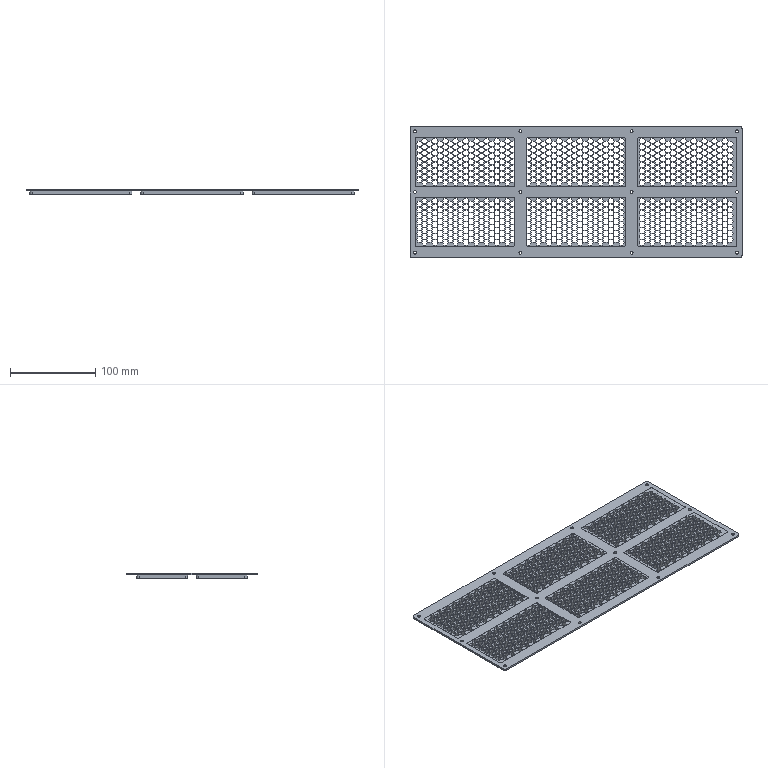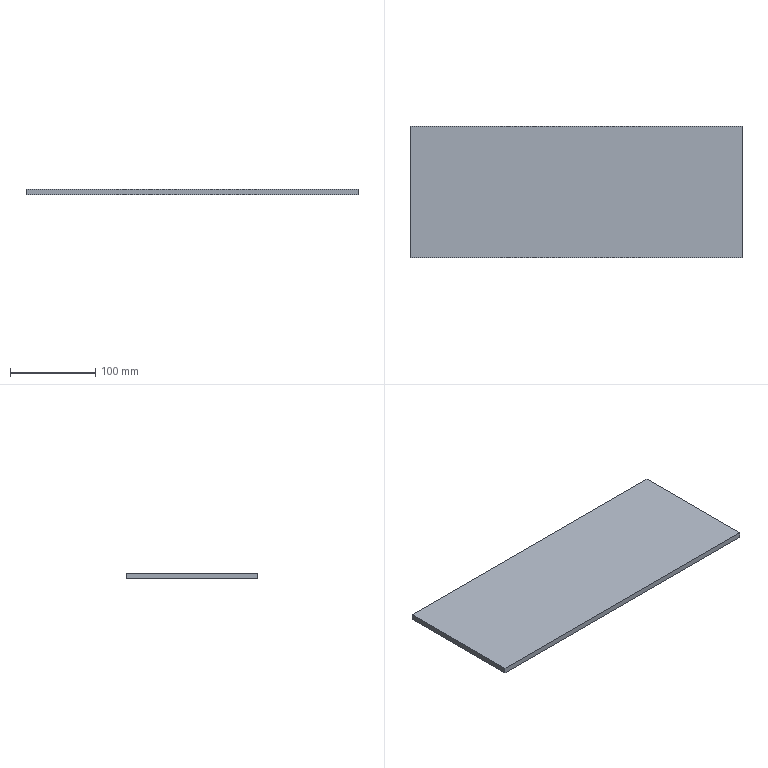CAM job | NX | 3-axis milling, drilling | stock box 388.5 x 153.5 x 6.5 mm
Tools:
number,name,description,diameter,corner_radius,flute_length,length,flutes
3,D2_FINISH,D2,2.0,0.0,6.0,50.0,2
12,D3_ROUGH,D3,3.0,0.0,9.0,50.0,2
0,D4_ROUGH,D4,4.0,0.0,12.0,50.0,2
2,D6_ROUGH,D6,6.0,0.0,16.0,60.0,2
2,D6_FINISH,D6,6.0,0.0,16.0,60.0,2
1,D80R0.8,方肩铣刀片,80.0,0.8,15.0,80.0,2
4,D4_CHAMFER,DJ4-32,4.0,0.0,2.0,50.0,2
0,Z2.5,Z2.5直柄钻头,2.5,0.0,30.0,57.0,2
5,Z3.5,Z3.5直柄钻头,3.5,0.0,39.0,70.0,2
0,M3X0.5,公制-铝用螺旋槽丝攻,2.5,0.0,11.0,18.0,2
6,D4,Drilling Tool,4.0,0.0,35.0,50.0,2
Operations, first 268 of 867 lines:
program,operation,operation_type,tool,method,geometry_group,spindle_rpm,surface_speed,feed_per_tooth,feed_cut,feed_plunge,cut_length_mm,path_length_mm,cut_time_min,machine_time_min
1,PLANAR_MILL,PlanarMilling,D80R0.8,METHOD,W1,3000.0,753.0,0.1667,1000.0,100.0,1521.0,2820.97,1.521,1.651
1,PLANAR_MILL_1,PlanarMilling,D6_ROUGH,METHOD,MCS_1,5500.0,100.0,0.1178,2000.0,100.0,18288.491,18394.491,9.144,9.155
1,PLANAR_MILL_1_COPY,PlanarMilling,D6_ROUGH,METHOD,MCS_1,4500.0,100.0,0.1178,800.0,100.0,2204.398,2316.398,2.756,2.767
1,FLOOR_FACING,VolumeBased25DMillingOperation,D6_ROUGH,METHOD,MCS_1,4500.0,100.0,0.1178,800.0,100.0,9696.176,10838.998,12.12,12.235
1,PLANAR_MILL_2,PlanarMilling,D2_FINISH,METHOD,MCS_1,4500.0,100.0,0.1178,600.0,100.0,2068.274,3272.854,3.447,3.568
1,PLANAR_MILL_1_COPY_COPY,PlanarMilling,D4_CHAMFER,METHOD,MCS_1,3500.0,100.0,0.1178,1000.0,100.0,1095.845,1193.845,1.096,1.106
1,DRILLING,Operation,D4_CHAMFER,METHOD,MCS_1,3000.0,0.0,0.0,200.0,0.0,57.0,1480.449,0.285,0.4273
1,DRILLING_COPY,Operation,Z3.5,METHOD,MCS_1,3000.0,0.0,0.0,200.0,0.0,108.0,1582.449,0.54,0.6874
2,DRILLING_COPY_1,Operation,D4_CHAMFER,METHOD,MCS_1,3000.0,0.0,0.0,200.0,0.0,4.75,69.7,0.0238,0.0302
2,DRILLING_COPY_1_COPY_1,Operation,D4_CHAMFER,METHOD,MCS_1,3000.0,0.0,0.0,200.0,0.0,4.75,69.7,0.0238,0.0302
2,DRILLING_COPY_1_COPY_2,Operation,D4_CHAMFER,METHOD,MCS_1,3000.0,0.0,0.0,200.0,0.0,4.75,69.7,0.0238,0.0302
2,DRILLING_COPY_1_COPY_3,Operation,D4_CHAMFER,METHOD,MCS_1,3000.0,0.0,0.0,200.0,0.0,4.75,69.7,0.0238,0.0302
2,DRILLING_COPY_1_COPY_4,Operation,D4_CHAMFER,METHOD,MCS_1,3000.0,0.0,0.0,200.0,0.0,4.75,69.7,0.0238,0.0302
2,DRILLING_COPY_1_COPY_5,Operation,D4_CHAMFER,METHOD,MCS_1,3000.0,0.0,0.0,200.0,0.0,4.75,69.7,0.0238,0.0302
2,DRILLING_COPY_1_COPY_6,Operation,D4_CHAMFER,METHOD,MCS_1,3000.0,0.0,0.0,200.0,0.0,4.75,69.7,0.0238,0.0302
2,DRILLING_COPY_1_COPY_7,Operation,D4_CHAMFER,METHOD,MCS_1,3000.0,0.0,0.0,200.0,0.0,4.75,69.7,0.0238,0.0302
2,DRILLING_COPY_1_COPY_8,Operation,D4_CHAMFER,METHOD,MCS_1,3000.0,0.0,0.0,200.0,0.0,4.75,69.7,0.0238,0.0302
2,DRILLING_COPY_1_COPY_9,Operation,D4_CHAMFER,METHOD,MCS_1,3000.0,0.0,0.0,200.0,0.0,4.75,69.7,0.0238,0.0302
2,DRILLING_COPY_1_COPY_1_COPY,Operation,D4_CHAMFER,METHOD,MCS_1,3000.0,0.0,0.0,200.0,0.0,4.75,69.7,0.0238,0.0302
2,DRILLING_COPY_1_COPY_2_COPY,Operation,D4_CHAMFER,METHOD,MCS_1,3000.0,0.0,0.0,200.0,0.0,4.75,69.7,0.0238,0.0302
2,DRILLING_COPY_1_COPY_3_COPY,Operation,D4_CHAMFER,METHOD,MCS_1,3000.0,0.0,0.0,200.0,0.0,4.75,69.7,0.0238,0.0302
2,DRILLING_COPY_1_COPY_4_COPY,Operation,D4_CHAMFER,METHOD,MCS_1,3000.0,0.0,0.0,200.0,0.0,4.75,69.7,0.0238,0.0302
2,DRILLING_COPY_1_COPY_5_COPY,Operation,D4_CHAMFER,METHOD,MCS_1,3000.0,0.0,0.0,200.0,0.0,4.75,69.7,0.0238,0.0302
2,DRILLING_COPY_1_COPY_6_COPY,Operation,D4_CHAMFER,METHOD,MCS_1,3000.0,0.0,0.0,200.0,0.0,4.75,69.7,0.0238,0.0302
2,DRILLING_COPY_1_COPY_7_COPY,Operation,D4_CHAMFER,METHOD,MCS_1,3000.0,0.0,0.0,200.0,0.0,4.75,69.7,0.0238,0.0302
2,DRILLING_COPY_1_COPY_8_COPY,Operation,D4_CHAMFER,METHOD,MCS_1,3000.0,0.0,0.0,200.0,0.0,4.75,69.7,0.0238,0.0302
2,DRILLING_COPY_1_COPY_10,Operation,D4_CHAMFER,METHOD,MCS_1,3000.0,0.0,0.0,200.0,0.0,4.75,69.7,0.0238,0.0302
2,DRILLING_COPY_1_COPY_1_COPY_1,Operation,D4_CHAMFER,METHOD,MCS_1,3000.0,0.0,0.0,200.0,0.0,4.75,69.7,0.0238,0.0302
2,DRILLING_COPY_1_COPY_2_COPY_1,Operation,D4_CHAMFER,METHOD,MCS_1,3000.0,0.0,0.0,200.0,0.0,4.75,69.7,0.0238,0.0302
2,DRILLING_COPY_1_COPY_3_COPY_1,Operation,D4_CHAMFER,METHOD,MCS_1,3000.0,0.0,0.0,200.0,0.0,4.75,69.7,0.0238,0.0302
2,DRILLING_COPY_1_COPY_4_COPY_1,Operation,D4_CHAMFER,METHOD,MCS_1,3000.0,0.0,0.0,200.0,0.0,4.75,69.7,0.0238,0.0302
2,DRILLING_COPY_1_COPY_5_COPY_1,Operation,D4_CHAMFER,METHOD,MCS_1,3000.0,0.0,0.0,200.0,0.0,4.75,69.7,0.0238,0.0302
2,DRILLING_COPY_1_COPY_6_COPY_1,Operation,D4_CHAMFER,METHOD,MCS_1,3000.0,0.0,0.0,200.0,0.0,4.75,69.7,0.0238,0.0302
2,DRILLING_COPY_1_COPY_7_COPY_1,Operation,D4_CHAMFER,METHOD,MCS_1,3000.0,0.0,0.0,200.0,0.0,4.75,69.7,0.0238,0.0302
2,DRILLING_COPY_1_COPY_8_COPY_1,Operation,D4_CHAMFER,METHOD,MCS_1,3000.0,0.0,0.0,200.0,0.0,4.75,69.7,0.0238,0.0302
2,DRILLING_COPY_1_COPY_11,Operation,D4_CHAMFER,METHOD,MCS_1,3000.0,0.0,0.0,200.0,0.0,4.75,69.7,0.0238,0.0302
2,DRILLING_COPY_1_COPY_1_COPY_2,Operation,D4_CHAMFER,METHOD,MCS_1,3000.0,0.0,0.0,200.0,0.0,4.75,69.7,0.0238,0.0302
2,DRILLING_COPY_1_COPY_2_COPY_2,Operation,D4_CHAMFER,METHOD,MCS_1,3000.0,0.0,0.0,200.0,0.0,4.75,69.7,0.0238,0.0302
2,DRILLING_COPY_1_COPY_3_COPY_2,Operation,D4_CHAMFER,METHOD,MCS_1,3000.0,0.0,0.0,200.0,0.0,4.75,69.7,0.0238,0.0302
2,DRILLING_COPY_1_COPY_4_COPY_2,Operation,D4_CHAMFER,METHOD,MCS_1,3000.0,0.0,0.0,200.0,0.0,4.75,69.7,0.0238,0.0302
2,DRILLING_COPY_1_COPY_5_COPY_2,Operation,D4_CHAMFER,METHOD,MCS_1,3000.0,0.0,0.0,200.0,0.0,4.75,69.7,0.0238,0.0302
2,DRILLING_COPY_1_COPY_6_COPY_2,Operation,D4_CHAMFER,METHOD,MCS_1,3000.0,0.0,0.0,200.0,0.0,4.75,69.7,0.0238,0.0302
2,DRILLING_COPY_1_COPY_7_COPY_2,Operation,D4_CHAMFER,METHOD,MCS_1,3000.0,0.0,0.0,200.0,0.0,4.75,69.7,0.0238,0.0302
2,DRILLING_COPY_1_COPY_8_COPY_2,Operation,D4_CHAMFER,METHOD,MCS_1,3000.0,0.0,0.0,200.0,0.0,4.75,69.7,0.0238,0.0302
2,DRILLING_COPY_1_COPY_12,Operation,D4_CHAMFER,METHOD,MCS_1,3000.0,0.0,0.0,200.0,0.0,4.75,69.7,0.0238,0.0302
2,DRILLING_COPY_1_COPY_1_COPY_3,Operation,D4_CHAMFER,METHOD,MCS_1,3000.0,0.0,0.0,200.0,0.0,4.75,69.7,0.0238,0.0302
2,DRILLING_COPY_1_COPY_2_COPY_3,Operation,D4_CHAMFER,METHOD,MCS_1,3000.0,0.0,0.0,200.0,0.0,4.75,69.7,0.0238,0.0302
2,DRILLING_COPY_1_COPY_3_COPY_3,Operation,D4_CHAMFER,METHOD,MCS_1,3000.0,0.0,0.0,200.0,0.0,4.75,69.7,0.0238,0.0302
2,DRILLING_COPY_1_COPY_4_COPY_3,Operation,D4_CHAMFER,METHOD,MCS_1,3000.0,0.0,0.0,200.0,0.0,4.75,69.7,0.0238,0.0302
2,DRILLING_COPY_1_COPY_5_COPY_3,Operation,D4_CHAMFER,METHOD,MCS_1,3000.0,0.0,0.0,200.0,0.0,4.75,69.7,0.0238,0.0302
2,DRILLING_COPY_1_COPY_6_COPY_3,Operation,D4_CHAMFER,METHOD,MCS_1,3000.0,0.0,0.0,200.0,0.0,4.75,69.7,0.0238,0.0302
2,DRILLING_COPY_1_COPY_7_COPY_3,Operation,D4_CHAMFER,METHOD,MCS_1,3000.0,0.0,0.0,200.0,0.0,4.75,69.7,0.0238,0.0302
2,DRILLING_COPY_1_COPY_8_COPY_3,Operation,D4_CHAMFER,METHOD,MCS_1,3000.0,0.0,0.0,200.0,0.0,4.75,69.7,0.0238,0.0302
2,DRILLING_COPY_1_COPY_13,Operation,D4_CHAMFER,METHOD,MCS_1,3000.0,0.0,0.0,200.0,0.0,4.75,69.7,0.0238,0.0302
2,DRILLING_COPY_1_COPY_1_COPY_4,Operation,D4_CHAMFER,METHOD,MCS_1,3000.0,0.0,0.0,200.0,0.0,4.75,69.7,0.0238,0.0302
2,DRILLING_COPY_1_COPY_2_COPY_4,Operation,D4_CHAMFER,METHOD,MCS_1,3000.0,0.0,0.0,200.0,0.0,4.75,69.7,0.0238,0.0302
2,DRILLING_COPY_1_COPY_3_COPY_4,Operation,D4_CHAMFER,METHOD,MCS_1,3000.0,0.0,0.0,200.0,0.0,4.75,69.7,0.0238,0.0302
2,DRILLING_COPY_1_COPY_4_COPY_4,Operation,D4_CHAMFER,METHOD,MCS_1,3000.0,0.0,0.0,200.0,0.0,4.75,69.7,0.0238,0.0302
2,DRILLING_COPY_1_COPY_5_COPY_4,Operation,D4_CHAMFER,METHOD,MCS_1,3000.0,0.0,0.0,200.0,0.0,4.75,69.7,0.0238,0.0302
2,DRILLING_COPY_1_COPY_6_COPY_4,Operation,D4_CHAMFER,METHOD,MCS_1,3000.0,0.0,0.0,200.0,0.0,4.75,69.7,0.0238,0.0302
2,DRILLING_COPY_1_COPY_7_COPY_4,Operation,D4_CHAMFER,METHOD,MCS_1,3000.0,0.0,0.0,200.0,0.0,4.75,69.7,0.0238,0.0302
2,DRILLING_COPY_1_COPY_8_COPY_4,Operation,D4_CHAMFER,METHOD,MCS_1,3000.0,0.0,0.0,200.0,0.0,4.75,69.7,0.0238,0.0302
2,DRILLING_COPY_1_COPY_14,Operation,D4_CHAMFER,METHOD,MCS_1,3000.0,0.0,0.0,200.0,0.0,4.75,69.7,0.0238,0.0302
2,DRILLING_COPY_1_COPY_1_COPY_5,Operation,D4_CHAMFER,METHOD,MCS_1,3000.0,0.0,0.0,200.0,0.0,4.75,69.7,0.0238,0.0302
2,DRILLING_COPY_1_COPY_2_COPY_5,Operation,D4_CHAMFER,METHOD,MCS_1,3000.0,0.0,0.0,200.0,0.0,4.75,69.7,0.0238,0.0302
2,DRILLING_COPY_1_COPY_3_COPY_5,Operation,D4_CHAMFER,METHOD,MCS_1,3000.0,0.0,0.0,200.0,0.0,4.75,69.7,0.0238,0.0302
2,DRILLING_COPY_1_COPY_4_COPY_5,Operation,D4_CHAMFER,METHOD,MCS_1,3000.0,0.0,0.0,200.0,0.0,4.75,69.7,0.0238,0.0302
2,DRILLING_COPY_1_COPY_5_COPY_5,Operation,D4_CHAMFER,METHOD,MCS_1,3000.0,0.0,0.0,200.0,0.0,4.75,69.7,0.0238,0.0302
2,DRILLING_COPY_1_COPY_6_COPY_5,Operation,D4_CHAMFER,METHOD,MCS_1,3000.0,0.0,0.0,200.0,0.0,4.75,69.7,0.0238,0.0302
2,DRILLING_COPY_1_COPY_7_COPY_5,Operation,D4_CHAMFER,METHOD,MCS_1,3000.0,0.0,0.0,200.0,0.0,4.75,69.7,0.0238,0.0302
2,DRILLING_COPY_1_COPY_8_COPY_5,Operation,D4_CHAMFER,METHOD,MCS_1,3000.0,0.0,0.0,200.0,0.0,4.75,69.7,0.0238,0.0302
2,DRILLING_COPY_1_COPY,Operation,D4_CHAMFER,METHOD,MCS_1,3000.0,0.0,0.0,200.0,0.0,4.75,69.7,0.0238,0.0302
2,DRILLING_COPY_1_COPY_COPY,Operation,D4_CHAMFER,METHOD,MCS_1,3000.0,0.0,0.0,200.0,0.0,4.75,69.7,0.0238,0.0302
2,DRILLING_COPY_1_COPY_COPY_1,Operation,D4_CHAMFER,METHOD,MCS_1,3000.0,0.0,0.0,200.0,0.0,4.75,69.7,0.0238,0.0302
2,DRILLING_COPY_1_COPY_COPY_2,Operation,D4_CHAMFER,METHOD,MCS_1,3000.0,0.0,0.0,200.0,0.0,4.75,69.7,0.0238,0.0302
2,DRILLING_COPY_1_COPY_COPY_3,Operation,D4_CHAMFER,METHOD,MCS_1,3000.0,0.0,0.0,200.0,0.0,4.75,69.7,0.0238,0.0302
2,DRILLING_COPY_1_COPY_COPY_4,Operation,D4_CHAMFER,METHOD,MCS_1,3000.0,0.0,0.0,200.0,0.0,4.75,69.7,0.0238,0.0302
2,DRILLING_COPY_1_COPY_COPY_5,Operation,D4_CHAMFER,METHOD,MCS_1,3000.0,0.0,0.0,200.0,0.0,4.75,69.7,0.0238,0.0302
2,DRILLING_COPY_1_COPY_COPY_6,Operation,D4_CHAMFER,METHOD,MCS_1,3000.0,0.0,0.0,200.0,0.0,4.75,69.7,0.0238,0.0302
2,DRILLING_COPY_1_COPY_COPY_7,Operation,D4_CHAMFER,METHOD,MCS_1,3000.0,0.0,0.0,200.0,0.0,4.75,69.7,0.0238,0.0302
2,DRILLING_COPY_1_COPY_COPY_8,Operation,D4_CHAMFER,METHOD,MCS_1,3000.0,0.0,0.0,200.0,0.0,4.75,69.7,0.0238,0.0302
2,DRILLING_COPY_1_COPY_COPY_COPY,Operation,D4_CHAMFER,METHOD,MCS_1,3000.0,0.0,0.0,200.0,0.0,4.75,69.7,0.0238,0.0302
2,DRILLING_COPY_1_COPY_COPY_1_COPY,Operation,D4_CHAMFER,METHOD,MCS_1,3000.0,0.0,0.0,200.0,0.0,4.75,69.7,0.0238,0.0302
2,DRILLING_COPY_1_COPY_COPY_2_COPY,Operation,D4_CHAMFER,METHOD,MCS_1,3000.0,0.0,0.0,200.0,0.0,4.75,69.7,0.0238,0.0302
2,DRILLING_COPY_1_COPY_COPY_3_COPY,Operation,D4_CHAMFER,METHOD,MCS_1,3000.0,0.0,0.0,200.0,0.0,4.75,69.7,0.0238,0.0302
2,DRILLING_COPY_1_COPY_COPY_4_COPY,Operation,D4_CHAMFER,METHOD,MCS_1,3000.0,0.0,0.0,200.0,0.0,4.75,69.7,0.0238,0.0302
2,DRILLING_COPY_1_COPY_COPY_5_COPY,Operation,D4_CHAMFER,METHOD,MCS_1,3000.0,0.0,0.0,200.0,0.0,4.75,69.7,0.0238,0.0302
2,DRILLING_COPY_1_COPY_COPY_6_COPY,Operation,D4_CHAMFER,METHOD,MCS_1,3000.0,0.0,0.0,200.0,0.0,4.75,69.7,0.0238,0.0302
2,DRILLING_COPY_1_COPY_COPY_7_COPY,Operation,D4_CHAMFER,METHOD,MCS_1,3000.0,0.0,0.0,200.0,0.0,4.75,69.7,0.0238,0.0302
2,DRILLING_COPY_1_COPY_COPY_9,Operation,D4_CHAMFER,METHOD,MCS_1,3000.0,0.0,0.0,200.0,0.0,4.75,69.7,0.0238,0.0302
2,DRILLING_COPY_1_COPY_COPY_COPY_1,Operation,D4_CHAMFER,METHOD,MCS_1,3000.0,0.0,0.0,200.0,0.0,4.75,69.7,0.0238,0.0302
2,DRILLING_COPY_1_COPY_COPY_1_COPY_1,Operation,D4_CHAMFER,METHOD,MCS_1,3000.0,0.0,0.0,200.0,0.0,4.75,69.7,0.0238,0.0302
2,DRILLING_COPY_1_COPY_COPY_2_COPY_1,Operation,D4_CHAMFER,METHOD,MCS_1,3000.0,0.0,0.0,200.0,0.0,4.75,69.7,0.0238,0.0302
2,DRILLING_COPY_1_COPY_COPY_3_COPY_1,Operation,D4_CHAMFER,METHOD,MCS_1,3000.0,0.0,0.0,200.0,0.0,4.75,69.7,0.0238,0.0302
2,DRILLING_COPY_1_COPY_COPY_4_COPY_1,Operation,D4_CHAMFER,METHOD,MCS_1,3000.0,0.0,0.0,200.0,0.0,4.75,69.7,0.0238,0.0302
2,DRILLING_COPY_1_COPY_COPY_5_COPY_1,Operation,D4_CHAMFER,METHOD,MCS_1,3000.0,0.0,0.0,200.0,0.0,4.75,69.7,0.0238,0.0302
2,DRILLING_COPY_1_COPY_COPY_6_COPY_1,Operation,D4_CHAMFER,METHOD,MCS_1,3000.0,0.0,0.0,200.0,0.0,4.75,69.7,0.0238,0.0302
2,DRILLING_COPY_1_COPY_COPY_7_COPY_1,Operation,D4_CHAMFER,METHOD,MCS_1,3000.0,0.0,0.0,200.0,0.0,4.75,69.7,0.0238,0.0302
2,DRILLING_COPY_1_COPY_COPY_10,Operation,D4_CHAMFER,METHOD,MCS_1,3000.0,0.0,0.0,200.0,0.0,4.75,69.7,0.0238,0.0302
2,DRILLING_COPY_1_COPY_COPY_COPY_2,Operation,D4_CHAMFER,METHOD,MCS_1,3000.0,0.0,0.0,200.0,0.0,4.75,69.7,0.0238,0.0302
2,DRILLING_COPY_1_COPY_COPY_1_COPY_2,Operation,D4_CHAMFER,METHOD,MCS_1,3000.0,0.0,0.0,200.0,0.0,4.75,69.7,0.0238,0.0302
2,DRILLING_COPY_1_COPY_COPY_2_COPY_2,Operation,D4_CHAMFER,METHOD,MCS_1,3000.0,0.0,0.0,200.0,0.0,4.75,69.7,0.0238,0.0302
2,DRILLING_COPY_1_COPY_COPY_3_COPY_2,Operation,D4_CHAMFER,METHOD,MCS_1,3000.0,0.0,0.0,200.0,0.0,4.75,69.7,0.0238,0.0302
2,DRILLING_COPY_1_COPY_COPY_4_COPY_2,Operation,D4_CHAMFER,METHOD,MCS_1,3000.0,0.0,0.0,200.0,0.0,4.75,69.7,0.0238,0.0302
2,DRILLING_COPY_1_COPY_COPY_5_COPY_2,Operation,D4_CHAMFER,METHOD,MCS_1,3000.0,0.0,0.0,200.0,0.0,4.75,69.7,0.0238,0.0302
2,DRILLING_COPY_1_COPY_COPY_6_COPY_2,Operation,D4_CHAMFER,METHOD,MCS_1,3000.0,0.0,0.0,200.0,0.0,4.75,69.7,0.0238,0.0302
2,DRILLING_COPY_1_COPY_COPY_7_COPY_2,Operation,D4_CHAMFER,METHOD,MCS_1,3000.0,0.0,0.0,200.0,0.0,4.75,69.7,0.0238,0.0302
2,DRILLING_COPY_1_COPY_COPY_11,Operation,D4_CHAMFER,METHOD,MCS_1,3000.0,0.0,0.0,200.0,0.0,4.75,69.7,0.0238,0.0302
2,DRILLING_COPY_1_COPY_COPY_COPY_3,Operation,D4_CHAMFER,METHOD,MCS_1,3000.0,0.0,0.0,200.0,0.0,4.75,69.7,0.0238,0.0302
2,DRILLING_COPY_1_COPY_COPY_1_COPY_3,Operation,D4_CHAMFER,METHOD,MCS_1,3000.0,0.0,0.0,200.0,0.0,4.75,69.7,0.0238,0.0302
2,DRILLING_COPY_1_COPY_COPY_2_COPY_3,Operation,D4_CHAMFER,METHOD,MCS_1,3000.0,0.0,0.0,200.0,0.0,4.75,69.7,0.0238,0.0302
2,DRILLING_COPY_1_COPY_COPY_3_COPY_3,Operation,D4_CHAMFER,METHOD,MCS_1,3000.0,0.0,0.0,200.0,0.0,4.75,69.7,0.0238,0.0302
2,DRILLING_COPY_1_COPY_COPY_4_COPY_3,Operation,D4_CHAMFER,METHOD,MCS_1,3000.0,0.0,0.0,200.0,0.0,4.75,69.7,0.0238,0.0302
2,DRILLING_COPY_1_COPY_COPY_5_COPY_3,Operation,D4_CHAMFER,METHOD,MCS_1,3000.0,0.0,0.0,200.0,0.0,4.75,69.7,0.0238,0.0302
2,DRILLING_COPY_1_COPY_COPY_6_COPY_3,Operation,D4_CHAMFER,METHOD,MCS_1,3000.0,0.0,0.0,200.0,0.0,4.75,69.7,0.0238,0.0302
2,DRILLING_COPY_1_COPY_COPY_7_COPY_3,Operation,D4_CHAMFER,METHOD,MCS_1,3000.0,0.0,0.0,200.0,0.0,4.75,69.7,0.0238,0.0302
2,DRILLING_COPY_1_COPY_COPY_12,Operation,D4_CHAMFER,METHOD,MCS_1,3000.0,0.0,0.0,200.0,0.0,4.75,69.7,0.0238,0.0302
2,DRILLING_COPY_1_COPY_COPY_COPY_4,Operation,D4_CHAMFER,METHOD,MCS_1,3000.0,0.0,0.0,200.0,0.0,4.75,69.7,0.0238,0.0302
2,DRILLING_COPY_1_COPY_COPY_1_COPY_4,Operation,D4_CHAMFER,METHOD,MCS_1,3000.0,0.0,0.0,200.0,0.0,4.75,69.7,0.0238,0.0302
2,DRILLING_COPY_1_COPY_COPY_2_COPY_4,Operation,D4_CHAMFER,METHOD,MCS_1,3000.0,0.0,0.0,200.0,0.0,4.75,69.7,0.0238,0.0302
2,DRILLING_COPY_1_COPY_COPY_3_COPY_4,Operation,D4_CHAMFER,METHOD,MCS_1,3000.0,0.0,0.0,200.0,0.0,4.75,69.7,0.0238,0.0302
2,DRILLING_COPY_1_COPY_COPY_4_COPY_4,Operation,D4_CHAMFER,METHOD,MCS_1,3000.0,0.0,0.0,200.0,0.0,4.75,69.7,0.0238,0.0302
2,DRILLING_COPY_1_COPY_COPY_5_COPY_4,Operation,D4_CHAMFER,METHOD,MCS_1,3000.0,0.0,0.0,200.0,0.0,4.75,69.7,0.0238,0.0302
2,DRILLING_COPY_1_COPY_COPY_6_COPY_4,Operation,D4_CHAMFER,METHOD,MCS_1,3000.0,0.0,0.0,200.0,0.0,4.75,69.7,0.0238,0.0302
2,DRILLING_COPY_1_COPY_COPY_7_COPY_4,Operation,D4_CHAMFER,METHOD,MCS_1,3000.0,0.0,0.0,200.0,0.0,4.75,69.7,0.0238,0.0302
2,DRILLING_COPY_1_COPY_COPY_13,Operation,D4_CHAMFER,METHOD,MCS_1,3000.0,0.0,0.0,200.0,0.0,4.75,69.7,0.0238,0.0302
2,DRILLING_COPY_1_COPY_COPY_COPY_5,Operation,D4_CHAMFER,METHOD,MCS_1,3000.0,0.0,0.0,200.0,0.0,4.75,69.7,0.0238,0.0302
2,DRILLING_COPY_1_COPY_COPY_1_COPY_5,Operation,D4_CHAMFER,METHOD,MCS_1,3000.0,0.0,0.0,200.0,0.0,4.75,69.7,0.0238,0.0302
2,DRILLING_COPY_1_COPY_COPY_2_COPY_5,Operation,D4_CHAMFER,METHOD,MCS_1,3000.0,0.0,0.0,200.0,0.0,4.75,69.7,0.0238,0.0302
2,DRILLING_COPY_1_COPY_COPY_3_COPY_5,Operation,D4_CHAMFER,METHOD,MCS_1,3000.0,0.0,0.0,200.0,0.0,4.75,69.7,0.0238,0.0302
2,DRILLING_COPY_1_COPY_COPY_4_COPY_5,Operation,D4_CHAMFER,METHOD,MCS_1,3000.0,0.0,0.0,200.0,0.0,4.75,69.7,0.0238,0.0302
2,DRILLING_COPY_1_COPY_COPY_5_COPY_5,Operation,D4_CHAMFER,METHOD,MCS_1,3000.0,0.0,0.0,200.0,0.0,4.75,69.7,0.0238,0.0302
2,DRILLING_COPY_1_COPY_COPY_6_COPY_5,Operation,D4_CHAMFER,METHOD,MCS_1,3000.0,0.0,0.0,200.0,0.0,4.75,69.7,0.0238,0.0302
2,DRILLING_COPY_1_COPY_COPY_7_COPY_5,Operation,D4_CHAMFER,METHOD,MCS_1,3000.0,0.0,0.0,200.0,0.0,4.75,69.7,0.0238,0.0302
2,DRILLING_COPY_1_COPY_COPY_14,Operation,D4_CHAMFER,METHOD,MCS_1,3000.0,0.0,0.0,200.0,0.0,4.75,69.7,0.0238,0.0302
2,DRILLING_COPY_1_COPY_COPY_COPY_6,Operation,D4_CHAMFER,METHOD,MCS_1,3000.0,0.0,0.0,200.0,0.0,4.75,69.7,0.0238,0.0302
2,DRILLING_COPY_1_COPY_COPY_1_COPY_6,Operation,D4_CHAMFER,METHOD,MCS_1,3000.0,0.0,0.0,200.0,0.0,4.75,69.7,0.0238,0.0302
2,DRILLING_COPY_1_COPY_COPY_2_COPY_6,Operation,D4_CHAMFER,METHOD,MCS_1,3000.0,0.0,0.0,200.0,0.0,4.75,69.7,0.0238,0.0302
2,DRILLING_COPY_1_COPY_COPY_3_COPY_6,Operation,D4_CHAMFER,METHOD,MCS_1,3000.0,0.0,0.0,200.0,0.0,4.75,69.7,0.0238,0.0302
2,DRILLING_COPY_1_COPY_COPY_4_COPY_6,Operation,D4_CHAMFER,METHOD,MCS_1,3000.0,0.0,0.0,200.0,0.0,4.75,69.7,0.0238,0.0302
2,DRILLING_COPY_1_COPY_COPY_5_COPY_6,Operation,D4_CHAMFER,METHOD,MCS_1,3000.0,0.0,0.0,200.0,0.0,4.75,69.7,0.0238,0.0302
2,DRILLING_COPY_1_COPY_COPY_6_COPY_6,Operation,D4_CHAMFER,METHOD,MCS_1,3000.0,0.0,0.0,200.0,0.0,4.75,69.7,0.0238,0.0302
2,DRILLING_COPY_1_COPY_COPY_7_COPY_6,Operation,D4_CHAMFER,METHOD,MCS_1,3000.0,0.0,0.0,200.0,0.0,4.75,69.7,0.0238,0.0302
2,DRILLING_COPY_1_COPY_15,Operation,D4_CHAMFER,METHOD,MCS_1,3000.0,0.0,0.0,200.0,0.0,4.75,69.7,0.0238,0.0302
2,DRILLING_COPY_1_COPY_15_COPY,Operation,D4_CHAMFER,METHOD,MCS_1,3000.0,0.0,0.0,200.0,0.0,4.75,69.7,0.0238,0.0302
2,DRILLING_COPY_1_COPY_15_COPY_1,Operation,D4_CHAMFER,METHOD,MCS_1,3000.0,0.0,0.0,200.0,0.0,4.75,69.7,0.0238,0.0302
2,DRILLING_COPY_1_COPY_15_COPY_2,Operation,D4_CHAMFER,METHOD,MCS_1,3000.0,0.0,0.0,200.0,0.0,4.75,69.7,0.0238,0.0302
2,DRILLING_COPY_1_COPY_15_COPY_3,Operation,D4_CHAMFER,METHOD,MCS_1,3000.0,0.0,0.0,200.0,0.0,4.75,69.7,0.0238,0.0302
2,DRILLING_COPY_1_COPY_15_COPY_4,Operation,D4_CHAMFER,METHOD,MCS_1,3000.0,0.0,0.0,200.0,0.0,4.75,69.7,0.0238,0.0302
2,DRILLING_COPY_1_COPY_15_COPY_5,Operation,D4_CHAMFER,METHOD,MCS_1,3000.0,0.0,0.0,200.0,0.0,4.75,69.7,0.0238,0.0302
3,DRILLING_COPY_1_COPY_15_COPY_6,Operation,D4_CHAMFER,METHOD,MCS_1,3000.0,0.0,0.0,200.0,0.0,4.75,69.7,0.0238,0.0302
3,DRILLING_COPY_1_COPY_15_COPY_6_COPY,Operation,D4_CHAMFER,METHOD,MCS_1,3000.0,0.0,0.0,200.0,0.0,4.75,69.7,0.0238,0.0302
3,DRILLING_COPY_1_COPY_15_COPY_6_COPY_1,Operation,D4_CHAMFER,METHOD,MCS_1,3000.0,0.0,0.0,200.0,0.0,4.75,69.7,0.0238,0.0302
3,DRILLING_COPY_1_COPY_15_COPY_6_COPY_2,Operation,D4_CHAMFER,METHOD,MCS_1,3000.0,0.0,0.0,200.0,0.0,4.75,69.7,0.0238,0.0302
3,DRILLING_COPY_1_COPY_15_COPY_6_COPY_3,Operation,D4_CHAMFER,METHOD,MCS_1,3000.0,0.0,0.0,200.0,0.0,4.75,69.7,0.0238,0.0302
3,DRILLING_COPY_1_COPY_15_COPY_6_COPY_4,Operation,D4_CHAMFER,METHOD,MCS_1,3000.0,0.0,0.0,200.0,0.0,4.75,69.7,0.0238,0.0302
3,DRILLING_COPY_1_COPY_15_COPY_6_COPY_5,Operation,D4_CHAMFER,METHOD,MCS_1,3000.0,0.0,0.0,200.0,0.0,4.75,69.7,0.0238,0.0302
3,DRILLING_COPY_1_COPY_15_COPY_6_COPY_6,Operation,D4_CHAMFER,METHOD,MCS_1,3000.0,0.0,0.0,200.0,0.0,4.75,69.7,0.0238,0.0302
3,DRILLING_COPY_1_COPY_15_COPY_6_COPY_COPY,Operation,D4_CHAMFER,METHOD,MCS_1,3000.0,0.0,0.0,200.0,0.0,4.75,69.7,0.0238,0.0302
3,DRILLING_COPY_1_COPY_15_COPY_6_COPY_1_COPY,Operation,D4_CHAMFER,METHOD,MCS_1,3000.0,0.0,0.0,200.0,0.0,4.75,69.7,0.0238,0.0302
3,DRILLING_COPY_1_COPY_15_COPY_6_COPY_2_COPY,Operation,D4_CHAMFER,METHOD,MCS_1,3000.0,0.0,0.0,200.0,0.0,4.75,69.7,0.0238,0.0302
3,DRILLING_COPY_1_COPY_15_COPY_6_COPY_3_COPY,Operation,D4_CHAMFER,METHOD,MCS_1,3000.0,0.0,0.0,200.0,0.0,4.75,69.7,0.0238,0.0302
3,DRILLING_COPY_1_COPY_15_COPY_6_COPY_4_COPY,Operation,D4_CHAMFER,METHOD,MCS_1,3000.0,0.0,0.0,200.0,0.0,4.75,69.7,0.0238,0.0302
3,DRILLING_COPY_1_COPY_15_COPY_6_COPY_5_COPY,Operation,D4_CHAMFER,METHOD,MCS_1,3000.0,0.0,0.0,200.0,0.0,4.75,69.7,0.0238,0.0302
3,DRILLING_COPY_1_COPY_15_COPY_6_COPY_7,Operation,D4_CHAMFER,METHOD,MCS_1,3000.0,0.0,0.0,200.0,0.0,4.75,69.7,0.0238,0.0302
3,DRILLING_COPY_1_COPY_15_COPY_6_COPY_COPY_1,Operation,D4_CHAMFER,METHOD,MCS_1,3000.0,0.0,0.0,200.0,0.0,4.75,69.7,0.0238,0.0302
3,DRILLING_COPY_1_COPY_15_COPY_6_COPY_1_COPY_1,Operation,D4_CHAMFER,METHOD,MCS_1,3000.0,0.0,0.0,200.0,0.0,4.75,69.7,0.0238,0.0302
3,DRILLING_COPY_1_COPY_15_COPY_6_COPY_2_COPY_1,Operation,D4_CHAMFER,METHOD,MCS_1,3000.0,0.0,0.0,200.0,0.0,4.75,69.7,0.0238,0.0302
3,DRILLING_COPY_1_COPY_15_COPY_6_COPY_3_COPY_1,Operation,D4_CHAMFER,METHOD,MCS_1,3000.0,0.0,0.0,200.0,0.0,4.75,69.7,0.0238,0.0302
3,DRILLING_COPY_1_COPY_15_COPY_6_COPY_4_COPY_1,Operation,D4_CHAMFER,METHOD,MCS_1,3000.0,0.0,0.0,200.0,0.0,4.75,69.7,0.0238,0.0302
3,DRILLING_COPY_1_COPY_15_COPY_6_COPY_5_COPY_1,Operation,D4_CHAMFER,METHOD,MCS_1,3000.0,0.0,0.0,200.0,0.0,4.75,69.7,0.0238,0.0302
3,DRILLING_COPY_1_COPY_15_COPY_6_COPY_8,Operation,D4_CHAMFER,METHOD,MCS_1,3000.0,0.0,0.0,200.0,0.0,4.75,69.7,0.0238,0.0302
3,DRILLING_COPY_1_COPY_15_COPY_6_COPY_COPY_2,Operation,D4_CHAMFER,METHOD,MCS_1,3000.0,0.0,0.0,200.0,0.0,4.75,69.7,0.0238,0.0302
3,DRILLING_COPY_1_COPY_15_COPY_6_COPY_1_COPY_2,Operation,D4_CHAMFER,METHOD,MCS_1,3000.0,0.0,0.0,200.0,0.0,4.75,69.7,0.0238,0.0302
3,DRILLING_COPY_1_COPY_15_COPY_6_COPY_2_COPY_2,Operation,D4_CHAMFER,METHOD,MCS_1,3000.0,0.0,0.0,200.0,0.0,4.75,69.7,0.0238,0.0302
3,DRILLING_COPY_1_COPY_15_COPY_6_COPY_3_COPY_2,Operation,D4_CHAMFER,METHOD,MCS_1,3000.0,0.0,0.0,200.0,0.0,4.75,69.7,0.0238,0.0302
3,DRILLING_COPY_1_COPY_15_COPY_6_COPY_4_COPY_2,Operation,D4_CHAMFER,METHOD,MCS_1,3000.0,0.0,0.0,200.0,0.0,4.75,69.7,0.0238,0.0302
3,DRILLING_COPY_1_COPY_15_COPY_6_COPY_5_COPY_2,Operation,D4_CHAMFER,METHOD,MCS_1,3000.0,0.0,0.0,200.0,0.0,4.75,69.7,0.0238,0.0302
3,DRILLING_COPY_1_COPY_15_COPY_6_COPY_9,Operation,D4_CHAMFER,METHOD,MCS_1,3000.0,0.0,0.0,200.0,0.0,4.75,69.7,0.0238,0.0302
3,DRILLING_COPY_1_COPY_15_COPY_6_COPY_COPY_3,Operation,D4_CHAMFER,METHOD,MCS_1,3000.0,0.0,0.0,200.0,0.0,4.75,69.7,0.0238,0.0302
3,DRILLING_COPY_1_COPY_15_COPY_6_COPY_1_COPY_3,Operation,D4_CHAMFER,METHOD,MCS_1,3000.0,0.0,0.0,200.0,0.0,4.75,69.7,0.0238,0.0302
3,DRILLING_COPY_1_COPY_15_COPY_6_COPY_2_COPY_3,Operation,D4_CHAMFER,METHOD,MCS_1,3000.0,0.0,0.0,200.0,0.0,4.75,69.7,0.0238,0.0302
3,DRILLING_COPY_1_COPY_15_COPY_6_COPY_3_COPY_3,Operation,D4_CHAMFER,METHOD,MCS_1,3000.0,0.0,0.0,200.0,0.0,4.75,69.7,0.0238,0.0302
3,DRILLING_COPY_1_COPY_15_COPY_6_COPY_4_COPY_3,Operation,D4_CHAMFER,METHOD,MCS_1,3000.0,0.0,0.0,200.0,0.0,4.75,69.7,0.0238,0.0302
3,DRILLING_COPY_1_COPY_15_COPY_6_COPY_5_COPY_3,Operation,D4_CHAMFER,METHOD,MCS_1,3000.0,0.0,0.0,200.0,0.0,4.75,69.7,0.0238,0.0302
3,DRILLING_COPY_1_COPY_15_COPY_6_COPY_10,Operation,D4_CHAMFER,METHOD,MCS_1,3000.0,0.0,0.0,200.0,0.0,4.75,69.7,0.0238,0.0302
3,DRILLING_COPY_1_COPY_15_COPY_6_COPY_COPY_4,Operation,D4_CHAMFER,METHOD,MCS_1,3000.0,0.0,0.0,200.0,0.0,4.75,69.7,0.0238,0.0302
3,DRILLING_COPY_1_COPY_15_COPY_6_COPY_1_COPY_4,Operation,D4_CHAMFER,METHOD,MCS_1,3000.0,0.0,0.0,200.0,0.0,4.75,69.7,0.0238,0.0302
3,DRILLING_COPY_1_COPY_15_COPY_6_COPY_2_COPY_4,Operation,D4_CHAMFER,METHOD,MCS_1,3000.0,0.0,0.0,200.0,0.0,4.75,69.7,0.0238,0.0302
3,DRILLING_COPY_1_COPY_15_COPY_6_COPY_3_COPY_4,Operation,D4_CHAMFER,METHOD,MCS_1,3000.0,0.0,0.0,200.0,0.0,4.75,69.7,0.0238,0.0302
3,DRILLING_COPY_1_COPY_15_COPY_6_COPY_4_COPY_4,Operation,D4_CHAMFER,METHOD,MCS_1,3000.0,0.0,0.0,200.0,0.0,4.75,69.7,0.0238,0.0302
3,DRILLING_COPY_1_COPY_15_COPY_6_COPY_5_COPY_4,Operation,D4_CHAMFER,METHOD,MCS_1,3000.0,0.0,0.0,200.0,0.0,4.75,69.7,0.0238,0.0302
3,DRILLING_COPY_1_COPY_15_COPY_6_COPY_11,Operation,D4_CHAMFER,METHOD,MCS_1,3000.0,0.0,0.0,200.0,0.0,4.75,69.7,0.0238,0.0302
3,DRILLING_COPY_1_COPY_15_COPY_6_COPY_COPY_5,Operation,D4_CHAMFER,METHOD,MCS_1,3000.0,0.0,0.0,200.0,0.0,4.75,69.7,0.0238,0.0302
3,DRILLING_COPY_1_COPY_15_COPY_6_COPY_1_COPY_5,Operation,D4_CHAMFER,METHOD,MCS_1,3000.0,0.0,0.0,200.0,0.0,4.75,69.7,0.0238,0.0302
3,DRILLING_COPY_1_COPY_15_COPY_6_COPY_2_COPY_5,Operation,D4_CHAMFER,METHOD,MCS_1,3000.0,0.0,0.0,200.0,0.0,4.75,69.7,0.0238,0.0302
3,DRILLING_COPY_1_COPY_15_COPY_6_COPY_3_COPY_5,Operation,D4_CHAMFER,METHOD,MCS_1,3000.0,0.0,0.0,200.0,0.0,4.75,69.7,0.0238,0.0302
3,DRILLING_COPY_1_COPY_15_COPY_6_COPY_4_COPY_5,Operation,D4_CHAMFER,METHOD,MCS_1,3000.0,0.0,0.0,200.0,0.0,4.75,69.7,0.0238,0.0302
3,DRILLING_COPY_1_COPY_15_COPY_6_COPY_5_COPY_5,Operation,D4_CHAMFER,METHOD,MCS_1,3000.0,0.0,0.0,200.0,0.0,4.75,69.7,0.0238,0.0302
3,DRILLING_COPY_1_COPY_15_COPY_6_COPY_12,Operation,D4_CHAMFER,METHOD,MCS_1,3000.0,0.0,0.0,200.0,0.0,4.75,69.7,0.0238,0.0302
3,DRILLING_COPY_1_COPY_15_COPY_6_COPY_COPY_6,Operation,D4_CHAMFER,METHOD,MCS_1,3000.0,0.0,0.0,200.0,0.0,4.75,69.7,0.0238,0.0302
3,DRILLING_COPY_1_COPY_15_COPY_6_COPY_1_COPY_6,Operation,D4_CHAMFER,METHOD,MCS_1,3000.0,0.0,0.0,200.0,0.0,4.75,69.7,0.0238,0.0302
3,DRILLING_COPY_1_COPY_15_COPY_6_COPY_2_COPY_6,Operation,D4_CHAMFER,METHOD,MCS_1,3000.0,0.0,0.0,200.0,0.0,4.75,69.7,0.0238,0.0302
3,DRILLING_COPY_1_COPY_15_COPY_6_COPY_3_COPY_6,Operation,D4_CHAMFER,METHOD,MCS_1,3000.0,0.0,0.0,200.0,0.0,4.75,69.7,0.0238,0.0302
3,DRILLING_COPY_1_COPY_15_COPY_6_COPY_4_COPY_6,Operation,D4_CHAMFER,METHOD,MCS_1,3000.0,0.0,0.0,200.0,0.0,4.75,69.7,0.0238,0.0302
3,DRILLING_COPY_1_COPY_15_COPY_6_COPY_5_COPY_6,Operation,D4_CHAMFER,METHOD,MCS_1,3000.0,0.0,0.0,200.0,0.0,4.75,69.7,0.0238,0.0302
3,DRILLING_COPY_1_COPY_15_COPY_6_COPY_13,Operation,D4_CHAMFER,METHOD,MCS_1,3000.0,0.0,0.0,200.0,0.0,4.75,69.7,0.0238,0.0302
3,DRILLING_COPY_1_COPY_15_COPY_6_COPY_COPY_7,Operation,D4_CHAMFER,METHOD,MCS_1,3000.0,0.0,0.0,200.0,0.0,4.75,69.7,0.0238,0.0302
3,DRILLING_COPY_1_COPY_15_COPY_6_COPY_1_COPY_7,Operation,D4_CHAMFER,METHOD,MCS_1,3000.0,0.0,0.0,200.0,0.0,4.75,69.7,0.0238,0.0302
3,DRILLING_COPY_1_COPY_15_COPY_6_COPY_2_COPY_7,Operation,D4_CHAMFER,METHOD,MCS_1,3000.0,0.0,0.0,200.0,0.0,4.75,69.7,0.0238,0.0302
3,DRILLING_COPY_1_COPY_15_COPY_6_COPY_3_COPY_7,Operation,D4_CHAMFER,METHOD,MCS_1,3000.0,0.0,0.0,200.0,0.0,4.75,69.7,0.0238,0.0302
3,DRILLING_COPY_1_COPY_15_COPY_6_COPY_4_COPY_7,Operation,D4_CHAMFER,METHOD,MCS_1,3000.0,0.0,0.0,200.0,0.0,4.75,69.7,0.0238,0.0302
3,DRILLING_COPY_1_COPY_15_COPY_6_COPY_5_COPY_7,Operation,D4_CHAMFER,METHOD,MCS_1,3000.0,0.0,0.0,200.0,0.0,4.75,69.7,0.0238,0.0302
3,DRILLING_COPY_1_COPY_15_COPY_6_COPY_14,Operation,D4_CHAMFER,METHOD,MCS_1,3000.0,0.0,0.0,200.0,0.0,4.75,69.7,0.0238,0.0302
3,DRILLING_COPY_1_COPY_15_COPY_6_COPY_COPY_8,Operation,D4_CHAMFER,METHOD,MCS_1,3000.0,0.0,0.0,200.0,0.0,4.75,69.7,0.0238,0.0302
3,DRILLING_COPY_1_COPY_15_COPY_6_COPY_1_COPY_8,Operation,D4_CHAMFER,METHOD,MCS_1,3000.0,0.0,0.0,200.0,0.0,4.75,69.7,0.0238,0.0302
3,DRILLING_COPY_1_COPY_15_COPY_6_COPY_2_COPY_8,Operation,D4_CHAMFER,METHOD,MCS_1,3000.0,0.0,0.0,200.0,0.0,4.75,69.7,0.0238,0.0302
3,DRILLING_COPY_1_COPY_15_COPY_6_COPY_3_COPY_8,Operation,D4_CHAMFER,METHOD,MCS_1,3000.0,0.0,0.0,200.0,0.0,4.75,69.7,0.0238,0.0302
3,DRILLING_COPY_1_COPY_15_COPY_6_COPY_4_COPY_8,Operation,D4_CHAMFER,METHOD,MCS_1,3000.0,0.0,0.0,200.0,0.0,4.75,69.7,0.0238,0.0302
3,DRILLING_COPY_1_COPY_15_COPY_6_COPY_5_COPY_8,Operation,D4_CHAMFER,METHOD,MCS_1,3000.0,0.0,0.0,200.0,0.0,4.75,69.7,0.0238,0.0302
3,DRILLING_COPY_1_COPY_15_COPY_6_COPY_15,Operation,D4_CHAMFER,METHOD,MCS_1,3000.0,0.0,0.0,200.0,0.0,4.75,69.7,0.0238,0.0302
3,DRILLING_COPY_1_COPY_15_COPY_6_COPY_15_COPY,Operation,D4_CHAMFER,METHOD,MCS_1,3000.0,0.0,0.0,200.0,0.0,4.75,69.7,0.0238,0.0302
3,DRILLING_COPY_1_COPY_15_COPY_6_COPY_15_COPY_1,Operation,D4_CHAMFER,METHOD,MCS_1,3000.0,0.0,0.0,200.0,0.0,4.75,69.7,0.0238,0.0302
3,DRILLING_COPY_1_COPY_15_COPY_6_COPY_15_COPY_2,Operation,D4_CHAMFER,METHOD,MCS_1,3000.0,0.0,0.0,200.0,0.0,4.75,69.7,0.0238,0.0302
3,DRILLING_COPY_1_COPY_15_COPY_6_COPY_15_COPY_3,Operation,D4_CHAMFER,METHOD,MCS_1,3000.0,0.0,0.0,200.0,0.0,4.75,69.7,0.0238,0.0302
3,DRILLING_COPY_1_COPY_15_COPY_6_COPY_15_COPY_4,Operation,D4_CHAMFER,METHOD,MCS_1,3000.0,0.0,0.0,200.0,0.0,4.75,69.7,0.0238,0.0302
3,DRILLING_COPY_1_COPY_15_COPY_6_COPY_15_COPY_5,Operation,D4_CHAMFER,METHOD,MCS_1,3000.0,0.0,0.0,200.0,0.0,4.75,69.7,0.0238,0.0302
3,DRILLING_COPY_1_COPY_15_COPY_6_COPY_15_COPY_6,Operation,D4_CHAMFER,METHOD,MCS_1,3000.0,0.0,0.0,200.0,0.0,4.75,69.7,0.0238,0.0302
3,DRILLING_COPY_1_COPY_15_COPY_6_COPY_15_COPY_7,Operation,D4_CHAMFER,METHOD,MCS_1,3000.0,0.0,0.0,200.0,0.0,4.75,69.7,0.0238,0.0302
3,DRILLING_COPY_1_COPY_15_COPY_6_COPY_15_COPY_8,Operation,D4_CHAMFER,METHOD,MCS_1,3000.0,0.0,0.0,200.0,0.0,4.75,69.7,0.0238,0.0302
3,DRILLING_COPY_1_COPY_15_COPY_6_COPY_15_COPY_COPY,Operation,D4_CHAMFER,METHOD,MCS_1,3000.0,0.0,0.0,200.0,0.0,4.75,69.7,0.0238,0.0302
3,DRILLING_COPY_1_COPY_15_COPY_6_COPY_15_COPY_1_COPY,Operation,D4_CHAMFER,METHOD,MCS_1,3000.0,0.0,0.0,200.0,0.0,4.75,69.7,0.0238,0.0302
3,DRILLING_COPY_1_COPY_15_COPY_6_COPY_15_COPY_2_COPY,Operation,D4_CHAMFER,METHOD,MCS_1,3000.0,0.0,0.0,200.0,0.0,4.75,69.7,0.0238,0.0302
3,DRILLING_COPY_1_COPY_15_COPY_6_COPY_15_COPY_3_COPY,Operation,D4_CHAMFER,METHOD,MCS_1,3000.0,0.0,0.0,200.0,0.0,4.75,69.7,0.0238,0.0302
3,DRILLING_COPY_1_COPY_15_COPY_6_COPY_15_COPY_4_COPY,Operation,D4_CHAMFER,METHOD,MCS_1,3000.0,0.0,0.0,200.0,0.0,4.75,69.7,0.0238,0.0302
3,DRILLING_COPY_1_COPY_15_COPY_6_COPY_15_COPY_5_COPY,Operation,D4_CHAMFER,METHOD,MCS_1,3000.0,0.0,0.0,200.0,0.0,4.75,69.7,0.0238,0.0302
3,DRILLING_COPY_1_COPY_15_COPY_6_COPY_15_COPY_6_COPY,Operation,D4_CHAMFER,METHOD,MCS_1,3000.0,0.0,0.0,200.0,0.0,4.75,69.7,0.0238,0.0302
3,DRILLING_COPY_1_COPY_15_COPY_6_COPY_15_COPY_7_COPY,Operation,D4_CHAMFER,METHOD,MCS_1,3000.0,0.0,0.0,200.0,0.0,4.75,69.7,0.0238,0.0302
3,DRILLING_COPY_1_COPY_15_COPY_6_COPY_15_COPY_9,Operation,D4_CHAMFER,METHOD,MCS_1,3000.0,0.0,0.0,200.0,0.0,4.75,69.7,0.0238,0.0302
3,DRILLING_COPY_1_COPY_15_COPY_6_COPY_15_COPY_COPY_1,Operation,D4_CHAMFER,METHOD,MCS_1,3000.0,0.0,0.0,200.0,0.0,4.75,69.7,0.0238,0.0302
3,DRILLING_COPY_1_COPY_15_COPY_6_COPY_15_COPY_1_COPY_1,Operation,D4_CHAMFER,METHOD,MCS_1,3000.0,0.0,0.0,200.0,0.0,4.75,69.7,0.0238,0.0302
3,DRILLING_COPY_1_COPY_15_COPY_6_COPY_15_COPY_2_COPY_1,Operation,D4_CHAMFER,METHOD,MCS_1,3000.0,0.0,0.0,200.0,0.0,4.75,69.7,0.0238,0.0302
3,DRILLING_COPY_1_COPY_15_COPY_6_COPY_15_COPY_3_COPY_1,Operation,D4_CHAMFER,METHOD,MCS_1,3000.0,0.0,0.0,200.0,0.0,4.75,69.7,0.0238,0.0302
3,DRILLING_COPY_1_COPY_15_COPY_6_COPY_15_COPY_4_COPY_1,Operation,D4_CHAMFER,METHOD,MCS_1,3000.0,0.0,0.0,200.0,0.0,4.75,69.7,0.0238,0.0302
3,DRILLING_COPY_1_COPY_15_COPY_6_COPY_15_COPY_5_COPY_1,Operation,D4_CHAMFER,METHOD,MCS_1,3000.0,0.0,0.0,200.0,0.0,4.75,69.7,0.0238,0.0302
3,DRILLING_COPY_1_COPY_15_COPY_6_COPY_15_COPY_6_COPY_1,Operation,D4_CHAMFER,METHOD,MCS_1,3000.0,0.0,0.0,200.0,0.0,4.75,69.7,0.0238,0.0302
3,DRILLING_COPY_1_COPY_15_COPY_6_COPY_15_COPY_7_COPY_1,Operation,D4_CHAMFER,METHOD,MCS_1,3000.0,0.0,0.0,200.0,0.0,4.75,69.7,0.0238,0.0302
3,DRILLING_COPY_1_COPY_15_COPY_6_COPY_15_COPY_10,Operation,D4_CHAMFER,METHOD,MCS_1,3000.0,0.0,0.0,200.0,0.0,4.75,69.7,0.0238,0.0302
3,DRILLING_COPY_1_COPY_15_COPY_6_COPY_15_COPY_COPY_2,Operation,D4_CHAMFER,METHOD,MCS_1,3000.0,0.0,0.0,200.0,0.0,4.75,69.7,0.0238,0.0302
3,DRILLING_COPY_1_COPY_15_COPY_6_COPY_15_COPY_1_COPY_2,Operation,D4_CHAMFER,METHOD,MCS_1,3000.0,0.0,0.0,200.0,0.0,4.75,69.7,0.0238,0.0302
3,DRILLING_COPY_1_COPY_15_COPY_6_COPY_15_COPY_2_COPY_2,Operation,D4_CHAMFER,METHOD,MCS_1,3000.0,0.0,0.0,200.0,0.0,4.75,69.7,0.0238,0.0302
3,DRILLING_COPY_1_COPY_15_COPY_6_COPY_15_COPY_3_COPY_2,Operation,D4_CHAMFER,METHOD,MCS_1,3000.0,0.0,0.0,200.0,0.0,4.75,69.7,0.0238,0.0302
3,DRILLING_COPY_1_COPY_15_COPY_6_COPY_15_COPY_4_COPY_2,Operation,D4_CHAMFER,METHOD,MCS_1,3000.0,0.0,0.0,200.0,0.0,4.75,69.7,0.0238,0.0302
3,DRILLING_COPY_1_COPY_15_COPY_6_COPY_15_COPY_5_COPY_2,Operation,D4_CHAMFER,METHOD,MCS_1,3000.0,0.0,0.0,200.0,0.0,4.75,69.7,0.0238,0.0302
3,DRILLING_COPY_1_COPY_15_COPY_6_COPY_15_COPY_6_COPY_2,Operation,D4_CHAMFER,METHOD,MCS_1,3000.0,0.0,0.0,200.0,0.0,4.75,69.7,0.0238,0.0302
3,DRILLING_COPY_1_COPY_15_COPY_6_COPY_15_COPY_7_COPY_2,Operation,D4_CHAMFER,METHOD,MCS_1,3000.0,0.0,0.0,200.0,0.0,4.75,69.7,0.0238,0.0302
3,DRILLING_COPY_1_COPY_15_COPY_6_COPY_15_COPY_11,Operation,D4_CHAMFER,METHOD,MCS_1,3000.0,0.0,0.0,200.0,0.0,4.75,69.7,0.0238,0.0302
3,DRILLING_COPY_1_COPY_15_COPY_6_COPY_15_COPY_COPY_3,Operation,D4_CHAMFER,METHOD,MCS_1,3000.0,0.0,0.0,200.0,0.0,4.75,69.7,0.0238,0.0302
3,DRILLING_COPY_1_COPY_15_COPY_6_COPY_15_COPY_1_COPY_3,Operation,D4_CHAMFER,METHOD,MCS_1,3000.0,0.0,0.0,200.0,0.0,4.75,69.7,0.0238,0.0302
3,DRILLING_COPY_1_COPY_15_COPY_6_COPY_15_COPY_2_COPY_3,Operation,D4_CHAMFER,METHOD,MCS_1,3000.0,0.0,0.0,200.0,0.0,4.75,69.7,0.0238,0.0302
3,DRILLING_COPY_1_COPY_15_COPY_6_COPY_15_COPY_3_COPY_3,Operation,D4_CHAMFER,METHOD,MCS_1,3000.0,0.0,0.0,200.0,0.0,4.75,69.7,0.0238,0.0302
3,DRILLING_COPY_1_COPY_15_COPY_6_COPY_15_COPY_4_COPY_3,Operation,D4_CHAMFER,METHOD,MCS_1,3000.0,0.0,0.0,200.0,0.0,4.75,69.7,0.0238,0.0302
3,DRILLING_COPY_1_COPY_15_COPY_6_COPY_15_COPY_5_COPY_3,Operation,D4_CHAMFER,METHOD,MCS_1,3000.0,0.0,0.0,200.0,0.0,4.75,69.7,0.0238,0.0302
3,DRILLING_COPY_1_COPY_15_COPY_6_COPY_15_COPY_6_COPY_3,Operation,D4_CHAMFER,METHOD,MCS_1,3000.0,0.0,0.0,200.0,0.0,4.75,69.7,0.0238,0.0302
3,DRILLING_COPY_1_COPY_15_COPY_6_COPY_15_COPY_7_COPY_3,Operation,D4_CHAMFER,METHOD,MCS_1,3000.0,0.0,0.0,200.0,0.0,4.75,69.7,0.0238,0.0302
3,DRILLING_COPY_1_COPY_15_COPY_6_COPY_15_COPY_12,Operation,D4_CHAMFER,METHOD,MCS_1,3000.0,0.0,0.0,200.0,0.0,4.75,69.7,0.0238,0.0302
3,DRILLING_COPY_1_COPY_15_COPY_6_COPY_15_COPY_COPY_4,Operation,D4_CHAMFER,METHOD,MCS_1,3000.0,0.0,0.0,200.0,0.0,4.75,69.7,0.0238,0.0302